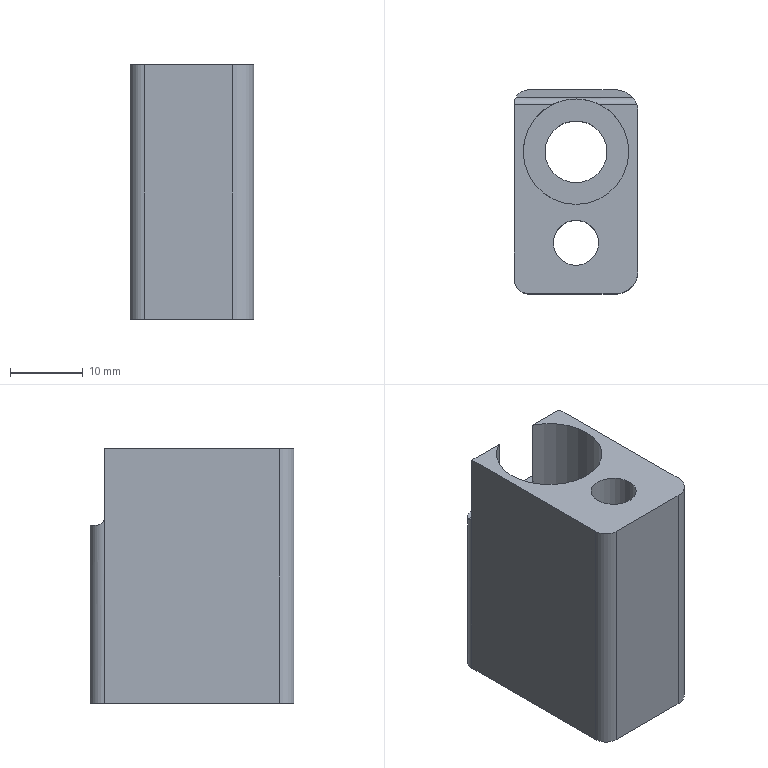Part | NX | features DIE-95 2 | 1 solid | 21 faces | box 17 x 28 x 35 mm | volume 11764 mm3 | plane 11 | cylinder 10 | commonest cylinder face diameters 4 x3 6 x2 2 x1 6.2 x1 8.5 x1 9 x1
STEP:
#1=CARTESIAN_POINT('',(4152.736,-820.122,848.216));
#2=VERTEX_POINT('',#1);
#3=CARTESIAN_POINT('',(4152.736,-820.123,858.716));
#4=VERTEX_POINT('',#3);
#5=CARTESIAN_POINT('',(4152.736,-820.123,848.216));
#6=CARTESIAN_POINT('',(4152.736,-820.123,851.716));
#7=CARTESIAN_POINT('',(4152.736,-820.123,855.216));
#8=CARTESIAN_POINT('',(4152.736,-820.123,858.716));
#9=B_SPLINE_CURVE_WITH_KNOTS('',3,(#5,#6,#7,#8),.UNSPECIFIED.,.F.,.F.,(4,4),(0.7,1.),.UNSPECIFIED.);
#10=EDGE_CURVE('',#2,#4,#9,.T.);
#11=ORIENTED_EDGE('',*,*,#10,.T.);
#12=CARTESIAN_POINT('',(4152.736,-820.122,858.716));
#13=VERTEX_POINT('',#12);
#14=CARTESIAN_POINT('',(4154.736,-820.123,858.716));
#15=DIRECTION('',(0.,0.,-1.));
#16=DIRECTION('',(1.,0.,0.));
#17=AXIS2_PLACEMENT_3D('',#14,#15,#16);
#18=CIRCLE('',#17,2.);
#19=EDGE_CURVE('',#13,#4,#18,.F.);
#20=ORIENTED_EDGE('',*,*,#19,.F.);
#21=CARTESIAN_POINT('',(4152.736,-820.122,849.216));
#22=VERTEX_POINT('',#21);
#23=CARTESIAN_POINT('',(4152.736,-820.122,823.716));
#24=DIRECTION('',(0.,0.,1.));
#25=VECTOR('',#24,1000.);
#26=LINE('',#23,#25);
#27=EDGE_CURVE('',#22,#13,#26,.T.);
#28=ORIENTED_EDGE('',*,*,#27,.F.);
#29=CARTESIAN_POINT('',(4152.736,-820.122,823.716));
#30=DIRECTION('',(0.,0.,1.));
#31=VECTOR('',#30,1000.);
#32=LINE('',#29,#31);
#33=EDGE_CURVE('',#2,#22,#32,.T.);
#34=ORIENTED_EDGE('',*,*,#33,.F.);
#35=EDGE_LOOP('',(#11,#20,#28,#34));
#36=FACE_BOUND('',#35,.T.);
#37=CARTESIAN_POINT('',(4154.736,-820.123,823.716));
#38=DIRECTION('',(0.,0.,1.));
#39=DIRECTION('',(1.,0.,0.));
#40=AXIS2_PLACEMENT_3D('',#37,#38,#39);
#41=CYLINDRICAL_SURFACE('',#40,2.);
#42=ADVANCED_FACE('',(#36),#41,.T.);
#43=ORIENTED_EDGE('',*,*,#27,.T.);
#44=CARTESIAN_POINT('',(4158.026,-820.122,858.716));
#45=VERTEX_POINT('',#44);
#46=CARTESIAN_POINT('',(3445.094,-820.122,858.716));
#47=DIRECTION('',(-1.,0.,0.));
#48=VECTOR('',#47,1000.);
#49=LINE('',#46,#48);
#50=EDGE_CURVE('',#13,#45,#49,.F.);
#51=ORIENTED_EDGE('',*,*,#50,.T.);
#52=CARTESIAN_POINT('',(4158.026,-820.122,849.216));
#53=VERTEX_POINT('',#52);
#54=CARTESIAN_POINT('',(4158.026,-820.122,847.716));
#55=DIRECTION('',(0.,0.,1.));
#56=VECTOR('',#55,1000.);
#57=LINE('',#54,#56);
#58=EDGE_CURVE('',#45,#53,#57,.F.);
#59=ORIENTED_EDGE('',*,*,#58,.T.);
#60=CARTESIAN_POINT('',(4155.381,-820.122,849.216));
#61=DIRECTION('',(-1.,0.,0.));
#62=VECTOR('',#61,1000.);
#63=LINE('',#60,#62);
#64=EDGE_CURVE('',#22,#53,#63,.F.);
#65=ORIENTED_EDGE('',*,*,#64,.F.);
#66=EDGE_LOOP('',(#43,#51,#59,#65));
#67=FACE_BOUND('',#66,.T.);
#68=CARTESIAN_POINT('',(4022.094,-820.122,867.716));
#69=DIRECTION('',(0.,-1.,0.));
#70=DIRECTION('',(0.,0.,1.));
#71=AXIS2_PLACEMENT_3D('',#68,#69,#70);
#72=PLANE('',#71);
#73=ADVANCED_FACE('',(#67),#72,.F.);
#74=CARTESIAN_POINT('',(4164.446,-820.122,849.216));
#75=VERTEX_POINT('',#74);
#76=CARTESIAN_POINT('',(4164.446,-820.122,858.716));
#77=VERTEX_POINT('',#76);
#78=CARTESIAN_POINT('',(4164.446,-820.122,847.716));
#79=DIRECTION('',(0.,0.,1.));
#80=VECTOR('',#79,1000.);
#81=LINE('',#78,#80);
#82=EDGE_CURVE('',#75,#77,#81,.T.);
#83=ORIENTED_EDGE('',*,*,#82,.T.);
#84=CARTESIAN_POINT('',(4169.564,-820.122,858.716));
#85=VERTEX_POINT('',#84);
#86=CARTESIAN_POINT('',(3445.094,-820.122,858.716));
#87=DIRECTION('',(-1.,0.,0.));
#88=VECTOR('',#87,1000.);
#89=LINE('',#86,#88);
#90=EDGE_CURVE('',#77,#85,#89,.F.);
#91=ORIENTED_EDGE('',*,*,#90,.T.);
#92=CARTESIAN_POINT('',(4169.564,-820.122,849.216));
#93=VERTEX_POINT('',#92);
#94=CARTESIAN_POINT('',(4169.564,-820.122,823.716));
#95=DIRECTION('',(0.,0.,1.));
#96=VECTOR('',#95,1000.);
#97=LINE('',#94,#96);
#98=EDGE_CURVE('',#85,#93,#97,.F.);
#99=ORIENTED_EDGE('',*,*,#98,.T.);
#100=CARTESIAN_POINT('',(4022.094,-820.122,849.216));
#101=DIRECTION('',(-1.,0.,0.));
#102=VECTOR('',#101,1000.);
#103=LINE('',#100,#102);
#104=EDGE_CURVE('',#75,#93,#103,.F.);
#105=ORIENTED_EDGE('',*,*,#104,.F.);
#106=EDGE_LOOP('',(#83,#91,#99,#105));
#107=FACE_BOUND('',#106,.T.);
#108=CARTESIAN_POINT('',(4022.094,-820.122,867.716));
#109=DIRECTION('',(0.,-1.,0.));
#110=DIRECTION('',(0.,0.,1.));
#111=AXIS2_PLACEMENT_3D('',#108,#109,#110);
#112=PLANE('',#111);
#113=ADVANCED_FACE('',(#107),#112,.F.);
#114=CARTESIAN_POINT('',(4169.736,-821.123,858.716));
#115=VERTEX_POINT('',#114);
#116=CARTESIAN_POINT('',(4166.736,-821.123,858.716));
#117=DIRECTION('',(0.,0.,-1.));
#118=DIRECTION('',(1.,0.,0.));
#119=AXIS2_PLACEMENT_3D('',#116,#117,#118);
#120=CIRCLE('',#119,3.);
#121=EDGE_CURVE('',#115,#85,#120,.F.);
#122=ORIENTED_EDGE('',*,*,#121,.F.);
#123=CARTESIAN_POINT('',(4169.736,-821.123,823.716));
#124=VERTEX_POINT('',#123);
#125=CARTESIAN_POINT('',(4169.736,-821.123,823.716));
#126=DIRECTION('',(0.,0.,1.));
#127=VECTOR('',#126,1000.);
#128=LINE('',#125,#127);
#129=EDGE_CURVE('',#115,#124,#128,.F.);
#130=ORIENTED_EDGE('',*,*,#129,.T.);
#131=CARTESIAN_POINT('',(4166.736,-818.123,823.716));
#132=VERTEX_POINT('',#131);
#133=CARTESIAN_POINT('',(4166.736,-821.123,823.716));
#134=DIRECTION('',(0.,0.,1.));
#135=DIRECTION('',(-1.,0.,0.));
#136=AXIS2_PLACEMENT_3D('',#133,#134,#135);
#137=CIRCLE('',#136,3.);
#138=EDGE_CURVE('',#124,#132,#137,.T.);
#139=ORIENTED_EDGE('',*,*,#138,.T.);
#140=CARTESIAN_POINT('',(4166.736,-818.123,848.216));
#141=VERTEX_POINT('',#140);
#142=CARTESIAN_POINT('',(4166.736,-818.123,823.716));
#143=DIRECTION('',(0.,0.,1.));
#144=VECTOR('',#143,1000.);
#145=LINE('',#142,#144);
#146=EDGE_CURVE('',#132,#141,#145,.T.);
#147=ORIENTED_EDGE('',*,*,#146,.T.);
#148=CARTESIAN_POINT('',(4168.972,-819.122,848.216));
#149=VERTEX_POINT('',#148);
#150=CARTESIAN_POINT('',(4166.736,-821.123,848.216));
#151=DIRECTION('',(0.,0.,-1.));
#152=DIRECTION('',(1.,0.,0.));
#153=AXIS2_PLACEMENT_3D('',#150,#151,#152);
#154=CIRCLE('',#153,3.);
#155=EDGE_CURVE('',#141,#149,#154,.T.);
#156=ORIENTED_EDGE('',*,*,#155,.T.);
#157=CARTESIAN_POINT('',(4169.564,-820.122,849.216));
#158=CARTESIAN_POINT('',(4169.564,-820.122,848.927));
#159=CARTESIAN_POINT('',(4169.481,-819.844,848.367));
#160=CARTESIAN_POINT('',(4169.164,-819.337,848.216));
#161=CARTESIAN_POINT('',(4168.972,-819.122,848.216));
#162=B_SPLINE_CURVE_WITH_KNOTS('',3,(#157,#158,#159,#160,#161),.UNSPECIFIED.,.F.,.F.,(4,1,4),(0.,0.0008558,0.001712),.UNSPECIFIED.);
#163=EDGE_CURVE('',#93,#149,#162,.T.);
#164=ORIENTED_EDGE('',*,*,#163,.F.);
#165=ORIENTED_EDGE('',*,*,#98,.F.);
#166=EDGE_LOOP('',(#122,#130,#139,#147,#156,#164,#165));
#167=FACE_BOUND('',#166,.T.);
#168=CARTESIAN_POINT('',(4166.736,-821.123,823.716));
#169=DIRECTION('',(0.,0.,1.));
#170=DIRECTION('',(1.,0.,0.));
#171=AXIS2_PLACEMENT_3D('',#168,#169,#170);
#172=CYLINDRICAL_SURFACE('',#171,3.);
#173=ADVANCED_FACE('',(#167),#172,.T.);
#174=CARTESIAN_POINT('',(4165.486,-826.623,823.716));
#175=VERTEX_POINT('',#174);
#176=CARTESIAN_POINT('',(4161.236,-826.623,823.716));
#177=DIRECTION('',(0.,0.,-1.));
#178=DIRECTION('',(1.,0.,0.));
#179=AXIS2_PLACEMENT_3D('',#176,#177,#178);
#180=CIRCLE('',#179,4.25);
#181=EDGE_CURVE('',#175,#175,#180,.F.);
#182=ORIENTED_EDGE('',*,*,#181,.T.);
#183=EDGE_LOOP('',(#182));
#184=FACE_BOUND('',#183,.T.);
#185=CARTESIAN_POINT('',(4165.736,-839.123,823.716));
#186=VERTEX_POINT('',#185);
#187=CARTESIAN_POINT('',(4161.236,-839.123,823.716));
#188=DIRECTION('',(0.,0.,-1.));
#189=DIRECTION('',(1.,0.,0.));
#190=AXIS2_PLACEMENT_3D('',#187,#188,#189);
#191=CIRCLE('',#190,4.5);
#192=EDGE_CURVE('',#186,#186,#191,.F.);
#193=ORIENTED_EDGE('',*,*,#192,.T.);
#194=EDGE_LOOP('',(#193));
#195=FACE_BOUND('',#194,.T.);
#196=ORIENTED_EDGE('',*,*,#138,.F.);
#197=CARTESIAN_POINT('',(4169.736,-843.123,823.716));
#198=VERTEX_POINT('',#197);
#199=CARTESIAN_POINT('',(4169.736,-839.123,823.716));
#200=DIRECTION('',(0.,1.,0.));
#201=VECTOR('',#200,1000.);
#202=LINE('',#199,#201);
#203=EDGE_CURVE('',#124,#198,#202,.F.);
#204=ORIENTED_EDGE('',*,*,#203,.T.);
#205=CARTESIAN_POINT('',(4166.736,-846.123,823.716));
#206=VERTEX_POINT('',#205);
#207=CARTESIAN_POINT('',(4166.736,-843.123,823.716));
#208=DIRECTION('',(0.,0.,1.));
#209=DIRECTION('',(-1.,0.,0.));
#210=AXIS2_PLACEMENT_3D('',#207,#208,#209);
#211=CIRCLE('',#210,3.);
#212=EDGE_CURVE('',#198,#206,#211,.F.);
#213=ORIENTED_EDGE('',*,*,#212,.T.);
#214=CARTESIAN_POINT('',(4154.736,-846.123,823.716));
#215=VERTEX_POINT('',#214);
#216=CARTESIAN_POINT('',(4161.236,-846.123,823.716));
#217=DIRECTION('',(-1.,0.,0.));
#218=VECTOR('',#217,1000.);
#219=LINE('',#216,#218);
#220=EDGE_CURVE('',#206,#215,#219,.T.);
#221=ORIENTED_EDGE('',*,*,#220,.T.);
#222=CARTESIAN_POINT('',(4152.736,-844.123,823.716));
#223=VERTEX_POINT('',#222);
#224=CARTESIAN_POINT('',(4154.736,-844.123,823.716));
#225=DIRECTION('',(0.,0.,1.));
#226=DIRECTION('',(-1.,0.,0.));
#227=AXIS2_PLACEMENT_3D('',#224,#225,#226);
#228=CIRCLE('',#227,2.);
#229=EDGE_CURVE('',#223,#215,#228,.T.);
#230=ORIENTED_EDGE('',*,*,#229,.F.);
#231=CARTESIAN_POINT('',(4152.736,-820.122,823.716));
#232=VERTEX_POINT('',#231);
#233=CARTESIAN_POINT('',(4152.736,-839.123,823.716));
#234=DIRECTION('',(0.,-1.,0.));
#235=VECTOR('',#234,1000.);
#236=LINE('',#233,#235);
#237=EDGE_CURVE('',#223,#232,#236,.F.);
#238=ORIENTED_EDGE('',*,*,#237,.T.);
#239=CARTESIAN_POINT('',(4154.736,-818.123,823.716));
#240=VERTEX_POINT('',#239);
#241=CARTESIAN_POINT('',(4154.736,-820.123,823.716));
#242=DIRECTION('',(0.,0.,1.));
#243=DIRECTION('',(-1.,0.,0.));
#244=AXIS2_PLACEMENT_3D('',#241,#242,#243);
#245=CIRCLE('',#244,2.);
#246=EDGE_CURVE('',#240,#232,#245,.T.);
#247=ORIENTED_EDGE('',*,*,#246,.F.);
#248=CARTESIAN_POINT('',(4161.236,-818.123,823.716));
#249=DIRECTION('',(-1.,0.,0.));
#250=VECTOR('',#249,1000.);
#251=LINE('',#248,#250);
#252=EDGE_CURVE('',#240,#132,#251,.F.);
#253=ORIENTED_EDGE('',*,*,#252,.T.);
#254=EDGE_LOOP('',(#196,#204,#213,#221,#230,#238,#247,#253));
#255=FACE_BOUND('',#254,.T.);
#256=CARTESIAN_POINT('',(3445.094,-717.123,823.716));
#257=DIRECTION('',(0.,0.,1.));
#258=DIRECTION('',(0.,-1.,0.));
#259=AXIS2_PLACEMENT_3D('',#256,#257,#258);
#260=PLANE('',#259);
#261=ADVANCED_FACE('',(#184,#195,#255),#260,.F.);
#262=CARTESIAN_POINT('',(4165.486,-826.623,847.716));
#263=VERTEX_POINT('',#262);
#264=CARTESIAN_POINT('',(4161.236,-826.623,847.716));
#265=DIRECTION('',(0.,0.,-1.));
#266=DIRECTION('',(1.,0.,0.));
#267=AXIS2_PLACEMENT_3D('',#264,#265,#266);
#268=CIRCLE('',#267,4.25);
#269=EDGE_CURVE('',#263,#263,#268,.T.);
#270=ORIENTED_EDGE('',*,*,#269,.T.);
#271=EDGE_LOOP('',(#270));
#272=FACE_BOUND('',#271,.T.);
#273=CARTESIAN_POINT('',(4161.236,-833.873,847.716));
#274=VERTEX_POINT('',#273);
#275=CARTESIAN_POINT('',(4161.236,-826.623,847.716));
#276=DIRECTION('',(0.,0.,-1.));
#277=DIRECTION('',(0.,-1.,0.));
#278=AXIS2_PLACEMENT_3D('',#275,#276,#277);
#279=CIRCLE('',#278,7.25);
#280=EDGE_CURVE('',#274,#274,#279,.F.);
#281=ORIENTED_EDGE('',*,*,#280,.T.);
#282=EDGE_LOOP('',(#281));
#283=FACE_BOUND('',#282,.T.);
#284=CARTESIAN_POINT('',(4161.236,-826.623,847.716));
#285=DIRECTION('',(0.,0.,1.));
#286=DIRECTION('',(1.,0.,0.));
#287=AXIS2_PLACEMENT_3D('',#284,#285,#286);
#288=PLANE('',#287);
#289=ADVANCED_FACE('',(#272,#283),#288,.T.);
#290=CARTESIAN_POINT('',(4164.336,-839.123,858.716));
#291=VERTEX_POINT('',#290);
#292=CARTESIAN_POINT('',(4161.236,-839.123,858.716));
#293=DIRECTION('',(0.,0.,-1.));
#294=DIRECTION('',(1.,0.,0.));
#295=AXIS2_PLACEMENT_3D('',#292,#293,#294);
#296=CIRCLE('',#295,3.1);
#297=EDGE_CURVE('',#291,#291,#296,.T.);
#298=ORIENTED_EDGE('',*,*,#297,.T.);
#299=EDGE_LOOP('',(#298));
#300=FACE_BOUND('',#299,.T.);
#301=ORIENTED_EDGE('',*,*,#90,.F.);
#302=CARTESIAN_POINT('',(4161.236,-826.623,858.716));
#303=DIRECTION('',(0.,0.,-1.));
#304=DIRECTION('',(1.,0.,0.));
#305=AXIS2_PLACEMENT_3D('',#302,#303,#304);
#306=CIRCLE('',#305,7.25);
#307=EDGE_CURVE('',#77,#45,#306,.T.);
#308=ORIENTED_EDGE('',*,*,#307,.T.);
#309=ORIENTED_EDGE('',*,*,#50,.F.);
#310=ORIENTED_EDGE('',*,*,#19,.T.);
#311=CARTESIAN_POINT('',(4152.736,-844.123,858.716));
#312=VERTEX_POINT('',#311);
#313=CARTESIAN_POINT('',(4152.736,-839.123,858.716));
#314=DIRECTION('',(0.,-1.,0.));
#315=VECTOR('',#314,1000.);
#316=LINE('',#313,#315);
#317=EDGE_CURVE('',#4,#312,#316,.T.);
#318=ORIENTED_EDGE('',*,*,#317,.T.);
#319=CARTESIAN_POINT('',(4154.736,-846.123,858.716));
#320=VERTEX_POINT('',#319);
#321=CARTESIAN_POINT('',(4154.736,-844.123,858.716));
#322=DIRECTION('',(0.,0.,-1.));
#323=DIRECTION('',(1.,0.,0.));
#324=AXIS2_PLACEMENT_3D('',#321,#322,#323);
#325=CIRCLE('',#324,2.);
#326=EDGE_CURVE('',#320,#312,#325,.T.);
#327=ORIENTED_EDGE('',*,*,#326,.F.);
#328=CARTESIAN_POINT('',(4166.736,-846.123,858.716));
#329=VERTEX_POINT('',#328);
#330=CARTESIAN_POINT('',(4161.236,-846.123,858.716));
#331=DIRECTION('',(1.,0.,0.));
#332=VECTOR('',#331,1000.);
#333=LINE('',#330,#332);
#334=EDGE_CURVE('',#320,#329,#333,.T.);
#335=ORIENTED_EDGE('',*,*,#334,.T.);
#336=CARTESIAN_POINT('',(4169.736,-843.123,858.716));
#337=VERTEX_POINT('',#336);
#338=CARTESIAN_POINT('',(4166.736,-843.123,858.716));
#339=DIRECTION('',(0.,0.,-1.));
#340=DIRECTION('',(1.,0.,0.));
#341=AXIS2_PLACEMENT_3D('',#338,#339,#340);
#342=CIRCLE('',#341,3.);
#343=EDGE_CURVE('',#329,#337,#342,.F.);
#344=ORIENTED_EDGE('',*,*,#343,.T.);
#345=CARTESIAN_POINT('',(4169.736,-839.123,858.716));
#346=DIRECTION('',(0.,1.,0.));
#347=VECTOR('',#346,1000.);
#348=LINE('',#345,#347);
#349=EDGE_CURVE('',#337,#115,#348,.T.);
#350=ORIENTED_EDGE('',*,*,#349,.T.);
#351=ORIENTED_EDGE('',*,*,#121,.T.);
#352=EDGE_LOOP('',(#301,#308,#309,#310,#318,#327,#335,#344,#350,#351));
#353=FACE_BOUND('',#352,.T.);
#354=CARTESIAN_POINT('',(3445.094,-717.123,858.716));
#355=DIRECTION('',(0.,0.,1.));
#356=DIRECTION('',(0.,-1.,0.));
#357=AXIS2_PLACEMENT_3D('',#354,#355,#356);
#358=PLANE('',#357);
#359=ADVANCED_FACE('',(#300,#353),#358,.T.);
#360=ORIENTED_EDGE('',*,*,#297,.F.);
#361=EDGE_LOOP('',(#360));
#362=FACE_BOUND('',#361,.T.);
#363=CARTESIAN_POINT('',(4158.136,-839.123,828.916));
#364=VERTEX_POINT('',#363);
#365=CARTESIAN_POINT('',(4161.236,-839.123,828.916));
#366=DIRECTION('',(0.,0.,1.));
#367=DIRECTION('',(-1.,0.,0.));
#368=AXIS2_PLACEMENT_3D('',#365,#366,#367);
#369=CIRCLE('',#368,3.1);
#370=EDGE_CURVE('',#364,#364,#369,.F.);
#371=ORIENTED_EDGE('',*,*,#370,.T.);
#372=EDGE_LOOP('',(#371));
#373=FACE_BOUND('',#372,.T.);
#374=CARTESIAN_POINT('',(4161.236,-839.123,823.716));
#375=DIRECTION('',(0.,0.,1.));
#376=DIRECTION('',(1.,0.,0.));
#377=AXIS2_PLACEMENT_3D('',#374,#375,#376);
#378=CYLINDRICAL_SURFACE('',#377,3.1);
#379=ADVANCED_FACE('',(#362,#373),#378,.F.);
#380=ORIENTED_EDGE('',*,*,#370,.F.);
#381=EDGE_LOOP('',(#380));
#382=FACE_BOUND('',#381,.T.);
#383=CARTESIAN_POINT('',(4156.736,-839.123,828.916));
#384=VERTEX_POINT('',#383);
#385=CARTESIAN_POINT('',(4161.236,-839.123,828.916));
#386=DIRECTION('',(0.,0.,1.));
#387=DIRECTION('',(-1.,0.,0.));
#388=AXIS2_PLACEMENT_3D('',#385,#386,#387);
#389=CIRCLE('',#388,4.5);
#390=EDGE_CURVE('',#384,#384,#389,.T.);
#391=ORIENTED_EDGE('',*,*,#390,.F.);
#392=EDGE_LOOP('',(#391));
#393=FACE_BOUND('',#392,.T.);
#394=CARTESIAN_POINT('',(4217.236,-839.123,828.916));
#395=DIRECTION('',(0.,0.,-1.));
#396=DIRECTION('',(-1.,0.,0.));
#397=AXIS2_PLACEMENT_3D('',#394,#395,#396);
#398=PLANE('',#397);
#399=ADVANCED_FACE('',(#382,#393),#398,.T.);
#400=ORIENTED_EDGE('',*,*,#390,.T.);
#401=EDGE_LOOP('',(#400));
#402=FACE_BOUND('',#401,.T.);
#403=ORIENTED_EDGE('',*,*,#192,.F.);
#404=EDGE_LOOP('',(#403));
#405=FACE_BOUND('',#404,.T.);
#406=CARTESIAN_POINT('',(4161.236,-839.123,823.716));
#407=DIRECTION('',(0.,0.,1.));
#408=DIRECTION('',(1.,0.,0.));
#409=AXIS2_PLACEMENT_3D('',#406,#407,#408);
#410=CYLINDRICAL_SURFACE('',#409,4.5);
#411=ADVANCED_FACE('',(#402,#405),#410,.F.);
#412=ORIENTED_EDGE('',*,*,#317,.F.);
#413=ORIENTED_EDGE('',*,*,#10,.F.);
#414=CARTESIAN_POINT('',(4152.736,-820.123,823.716));
#415=CARTESIAN_POINT('',(4152.736,-820.123,831.883));
#416=CARTESIAN_POINT('',(4152.736,-820.123,840.05));
#417=CARTESIAN_POINT('',(4152.736,-820.123,848.216));
#418=B_SPLINE_CURVE_WITH_KNOTS('',3,(#414,#415,#416,#417),.UNSPECIFIED.,.F.,.F.,(4,4),(0.,0.7),.UNSPECIFIED.);
#419=EDGE_CURVE('',#232,#2,#418,.T.);
#420=ORIENTED_EDGE('',*,*,#419,.F.);
#421=ORIENTED_EDGE('',*,*,#237,.F.);
#422=CARTESIAN_POINT('',(4152.736,-844.123,823.716));
#423=DIRECTION('',(0.,0.,1.));
#424=VECTOR('',#423,1000.);
#425=LINE('',#422,#424);
#426=EDGE_CURVE('',#312,#223,#425,.F.);
#427=ORIENTED_EDGE('',*,*,#426,.F.);
#428=EDGE_LOOP('',(#412,#413,#420,#421,#427));
#429=FACE_BOUND('',#428,.T.);
#430=CARTESIAN_POINT('',(4152.736,-839.123,823.716));
#431=DIRECTION('',(-1.,0.,0.));
#432=DIRECTION('',(0.,0.,1.));
#433=AXIS2_PLACEMENT_3D('',#430,#431,#432);
#434=PLANE('',#433);
#435=ADVANCED_FACE('',(#429),#434,.T.);
#436=ORIENTED_EDGE('',*,*,#220,.F.);
#437=CARTESIAN_POINT('',(4166.736,-846.123,823.716));
#438=DIRECTION('',(0.,0.,1.));
#439=VECTOR('',#438,1000.);
#440=LINE('',#437,#439);
#441=EDGE_CURVE('',#329,#206,#440,.F.);
#442=ORIENTED_EDGE('',*,*,#441,.F.);
#443=ORIENTED_EDGE('',*,*,#334,.F.);
#444=CARTESIAN_POINT('',(4154.736,-846.123,823.716));
#445=DIRECTION('',(0.,0.,1.));
#446=VECTOR('',#445,1000.);
#447=LINE('',#444,#446);
#448=EDGE_CURVE('',#215,#320,#447,.T.);
#449=ORIENTED_EDGE('',*,*,#448,.F.);
#450=EDGE_LOOP('',(#436,#442,#443,#449));
#451=FACE_BOUND('',#450,.T.);
#452=CARTESIAN_POINT('',(4161.236,-846.123,823.716));
#453=DIRECTION('',(0.,-1.,0.));
#454=DIRECTION('',(0.,0.,1.));
#455=AXIS2_PLACEMENT_3D('',#452,#453,#454);
#456=PLANE('',#455);
#457=ADVANCED_FACE('',(#451),#456,.T.);
#458=ORIENTED_EDGE('',*,*,#203,.F.);
#459=ORIENTED_EDGE('',*,*,#129,.F.);
#460=ORIENTED_EDGE('',*,*,#349,.F.);
#461=CARTESIAN_POINT('',(4169.736,-843.123,823.716));
#462=DIRECTION('',(0.,0.,1.));
#463=VECTOR('',#462,1000.);
#464=LINE('',#461,#463);
#465=EDGE_CURVE('',#198,#337,#464,.T.);
#466=ORIENTED_EDGE('',*,*,#465,.F.);
#467=EDGE_LOOP('',(#458,#459,#460,#466));
#468=FACE_BOUND('',#467,.T.);
#469=CARTESIAN_POINT('',(4169.736,-839.123,823.716));
#470=DIRECTION('',(1.,0.,0.));
#471=DIRECTION('',(0.,0.,-1.));
#472=AXIS2_PLACEMENT_3D('',#469,#470,#471);
#473=PLANE('',#472);
#474=ADVANCED_FACE('',(#468),#473,.T.);
#475=ORIENTED_EDGE('',*,*,#212,.F.);
#476=ORIENTED_EDGE('',*,*,#465,.T.);
#477=ORIENTED_EDGE('',*,*,#343,.F.);
#478=ORIENTED_EDGE('',*,*,#441,.T.);
#479=EDGE_LOOP('',(#475,#476,#477,#478));
#480=FACE_BOUND('',#479,.T.);
#481=CARTESIAN_POINT('',(4166.736,-843.123,823.716));
#482=DIRECTION('',(0.,0.,1.));
#483=DIRECTION('',(1.,0.,0.));
#484=AXIS2_PLACEMENT_3D('',#481,#482,#483);
#485=CYLINDRICAL_SURFACE('',#484,3.);
#486=ADVANCED_FACE('',(#480),#485,.T.);
#487=ORIENTED_EDGE('',*,*,#229,.T.);
#488=ORIENTED_EDGE('',*,*,#448,.T.);
#489=ORIENTED_EDGE('',*,*,#326,.T.);
#490=ORIENTED_EDGE('',*,*,#426,.T.);
#491=EDGE_LOOP('',(#487,#488,#489,#490));
#492=FACE_BOUND('',#491,.T.);
#493=CARTESIAN_POINT('',(4154.736,-844.123,823.716));
#494=DIRECTION('',(0.,0.,1.));
#495=DIRECTION('',(1.,0.,0.));
#496=AXIS2_PLACEMENT_3D('',#493,#494,#495);
#497=CYLINDRICAL_SURFACE('',#496,2.);
#498=ADVANCED_FACE('',(#492),#497,.T.);
#499=ORIENTED_EDGE('',*,*,#181,.F.);
#500=EDGE_LOOP('',(#499));
#501=FACE_BOUND('',#500,.T.);
#502=ORIENTED_EDGE('',*,*,#269,.F.);
#503=EDGE_LOOP('',(#502));
#504=FACE_BOUND('',#503,.T.);
#505=CARTESIAN_POINT('',(4161.236,-826.623,822.716));
#506=DIRECTION('',(0.,0.,1.));
#507=DIRECTION('',(1.,0.,0.));
#508=AXIS2_PLACEMENT_3D('',#505,#506,#507);
#509=CYLINDRICAL_SURFACE('',#508,4.25);
#510=ADVANCED_FACE('',(#501,#504),#509,.F.);
#511=ORIENTED_EDGE('',*,*,#280,.F.);
#512=EDGE_LOOP('',(#511));
#513=FACE_BOUND('',#512,.T.);
#514=ORIENTED_EDGE('',*,*,#307,.F.);
#515=ORIENTED_EDGE('',*,*,#82,.F.);
#516=CARTESIAN_POINT('',(4158.026,-820.122,849.216));
#517=CARTESIAN_POINT('',(4158.026,-820.122,848.901));
#518=CARTESIAN_POINT('',(4158.562,-819.862,848.49));
#519=CARTESIAN_POINT('',(4159.407,-819.588,848.324));
#520=CARTESIAN_POINT('',(4160.321,-819.411,848.256));
#521=CARTESIAN_POINT('',(4161.23,-819.354,848.244));
#522=CARTESIAN_POINT('',(4162.156,-819.411,848.256));
#523=CARTESIAN_POINT('',(4163.064,-819.588,848.323));
#524=CARTESIAN_POINT('',(4163.912,-819.862,848.492));
#525=CARTESIAN_POINT('',(4164.446,-820.122,848.9));
#526=CARTESIAN_POINT('',(4164.446,-820.122,849.216));
#527=B_SPLINE_CURVE_WITH_KNOTS('',3,(#516,#517,#518,#519,#520,#521,#522,#523,#524,#525,#526),.UNSPECIFIED.,.F.,.F.,(4,1,1,1,1,1,1,1,4),(0.,0.0009304,0.001861,0.002791,0.003722,0.004652,0.005582,0.006513,0.007443),.UNSPECIFIED.);
#528=EDGE_CURVE('',#53,#75,#527,.T.);
#529=ORIENTED_EDGE('',*,*,#528,.F.);
#530=ORIENTED_EDGE('',*,*,#58,.F.);
#531=EDGE_LOOP('',(#514,#515,#529,#530));
#532=FACE_BOUND('',#531,.T.);
#533=CARTESIAN_POINT('',(4161.236,-826.623,847.716));
#534=DIRECTION('',(0.,0.,1.));
#535=DIRECTION('',(1.,0.,0.));
#536=AXIS2_PLACEMENT_3D('',#533,#534,#535);
#537=CYLINDRICAL_SURFACE('',#536,7.25);
#538=ADVANCED_FACE('',(#513,#532),#537,.F.);
#539=CARTESIAN_POINT('',(4154.736,-818.123,848.216));
#540=VERTEX_POINT('',#539);
#541=CARTESIAN_POINT('',(4161.236,-818.123,848.216));
#542=DIRECTION('',(1.,0.,0.));
#543=VECTOR('',#542,1000.);
#544=LINE('',#541,#543);
#545=EDGE_CURVE('',#540,#141,#544,.T.);
#546=ORIENTED_EDGE('',*,*,#545,.T.);
#547=ORIENTED_EDGE('',*,*,#146,.F.);
#548=ORIENTED_EDGE('',*,*,#252,.F.);
#549=CARTESIAN_POINT('',(4154.736,-818.123,823.716));
#550=DIRECTION('',(0.,0.,1.));
#551=VECTOR('',#550,1000.);
#552=LINE('',#549,#551);
#553=EDGE_CURVE('',#540,#240,#552,.F.);
#554=ORIENTED_EDGE('',*,*,#553,.F.);
#555=EDGE_LOOP('',(#546,#547,#548,#554));
#556=FACE_BOUND('',#555,.T.);
#557=CARTESIAN_POINT('',(4161.236,-818.123,823.716));
#558=DIRECTION('',(0.,1.,0.));
#559=DIRECTION('',(0.,0.,-1.));
#560=AXIS2_PLACEMENT_3D('',#557,#558,#559);
#561=PLANE('',#560);
#562=ADVANCED_FACE('',(#556),#561,.T.);
#563=ORIENTED_EDGE('',*,*,#155,.F.);
#564=ORIENTED_EDGE('',*,*,#545,.F.);
#565=CARTESIAN_POINT('',(4153.004,-819.122,848.216));
#566=VERTEX_POINT('',#565);
#567=CARTESIAN_POINT('',(4154.736,-820.123,848.216));
#568=DIRECTION('',(0.,0.,-1.));
#569=DIRECTION('',(1.,0.,0.));
#570=AXIS2_PLACEMENT_3D('',#567,#568,#569);
#571=CIRCLE('',#570,2.);
#572=EDGE_CURVE('',#566,#540,#571,.T.);
#573=ORIENTED_EDGE('',*,*,#572,.F.);
#574=CARTESIAN_POINT('',(4161.236,-819.122,848.216));
#575=DIRECTION('',(-1.,0.,0.));
#576=VECTOR('',#575,1000.);
#577=LINE('',#574,#576);
#578=EDGE_CURVE('',#149,#566,#577,.T.);
#579=ORIENTED_EDGE('',*,*,#578,.F.);
#580=EDGE_LOOP('',(#563,#564,#573,#579));
#581=FACE_BOUND('',#580,.T.);
#582=CARTESIAN_POINT('',(4161.236,-826.623,848.216));
#583=DIRECTION('',(0.,0.,1.));
#584=DIRECTION('',(1.,0.,0.));
#585=AXIS2_PLACEMENT_3D('',#582,#583,#584);
#586=PLANE('',#585);
#587=ADVANCED_FACE('',(#581),#586,.T.);
#588=ORIENTED_EDGE('',*,*,#419,.T.);
#589=ORIENTED_EDGE('',*,*,#33,.T.);
#590=CARTESIAN_POINT('',(4153.004,-819.122,848.216));
#591=CARTESIAN_POINT('',(4152.733,-819.592,848.216));
#592=CARTESIAN_POINT('',(4152.736,-820.122,848.673));
#593=CARTESIAN_POINT('',(4152.736,-820.122,849.216));
#594=B_SPLINE_CURVE_WITH_KNOTS('',3,(#590,#591,#592,#593),.UNSPECIFIED.,.F.,.F.,(4,4),(0.,0.001608),.UNSPECIFIED.);
#595=EDGE_CURVE('',#566,#22,#594,.T.);
#596=ORIENTED_EDGE('',*,*,#595,.F.);
#597=ORIENTED_EDGE('',*,*,#572,.T.);
#598=ORIENTED_EDGE('',*,*,#553,.T.);
#599=ORIENTED_EDGE('',*,*,#246,.T.);
#600=EDGE_LOOP('',(#588,#589,#596,#597,#598,#599));
#601=FACE_BOUND('',#600,.T.);
#602=CARTESIAN_POINT('',(4154.736,-820.123,823.716));
#603=DIRECTION('',(0.,0.,1.));
#604=DIRECTION('',(1.,0.,0.));
#605=AXIS2_PLACEMENT_3D('',#602,#603,#604);
#606=CYLINDRICAL_SURFACE('',#605,2.);
#607=ADVANCED_FACE('',(#601),#606,.T.);
#608=ORIENTED_EDGE('',*,*,#163,.T.);
#609=ORIENTED_EDGE('',*,*,#578,.T.);
#610=ORIENTED_EDGE('',*,*,#595,.T.);
#611=ORIENTED_EDGE('',*,*,#64,.T.);
#612=ORIENTED_EDGE('',*,*,#528,.T.);
#613=ORIENTED_EDGE('',*,*,#104,.T.);
#614=EDGE_LOOP('',(#608,#609,#610,#611,#612,#613));
#615=FACE_BOUND('',#614,.T.);
#616=CARTESIAN_POINT('',(4161.236,-819.122,849.216));
#617=DIRECTION('',(-1.,0.,0.));
#618=DIRECTION('',(0.,0.,1.));
#619=AXIS2_PLACEMENT_3D('',#616,#617,#618);
#620=CYLINDRICAL_SURFACE('',#619,1.);
#621=ADVANCED_FACE('',(#615),#620,.F.);
#622=CLOSED_SHELL('',(#42,#73,#113,#173,#261,#289,#359,#379,#399,#411,#435,#457,#474,#486,#498,#510,#538,#562,#587,#607,#621));
#623=MANIFOLD_SOLID_BREP('',#622);
#624=(LENGTH_UNIT()NAMED_UNIT(*)SI_UNIT(.MILLI.,.METRE.));
#625=UNCERTAINTY_MEASURE_WITH_UNIT(LENGTH_MEASURE(0.0508),#624,'','');
#626=(NAMED_UNIT(*)PLANE_ANGLE_UNIT()SI_UNIT($,.RADIAN.));
#627=(NAMED_UNIT(*)SI_UNIT($,.STERADIAN.)SOLID_ANGLE_UNIT());
#628=(GEOMETRIC_REPRESENTATION_CONTEXT(3)GLOBAL_UNCERTAINTY_ASSIGNED_CONTEXT((#625))GLOBAL_UNIT_ASSIGNED_CONTEXT((#624,#626,#627))REPRESENTATION_CONTEXT('',''));
#629=ADVANCED_BREP_SHAPE_REPRESENTATION('',(#623),#628);